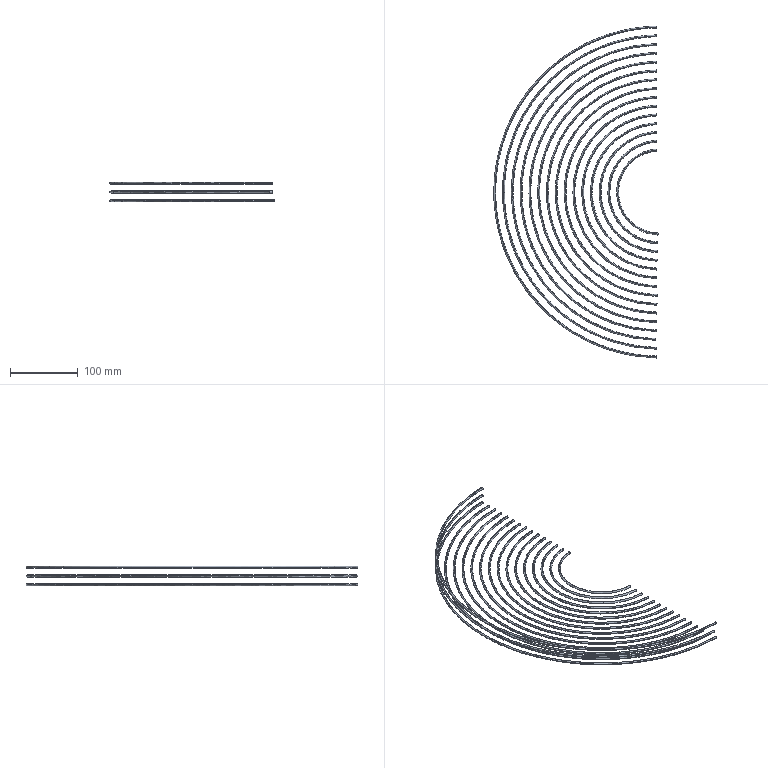Part | SolidWorks | features BaseBody 17 | 17 solids | 113 faces | box 243.22 x 490.896 x 29.005 mm | volume 60608 mm3 | spline 79 | plane 34